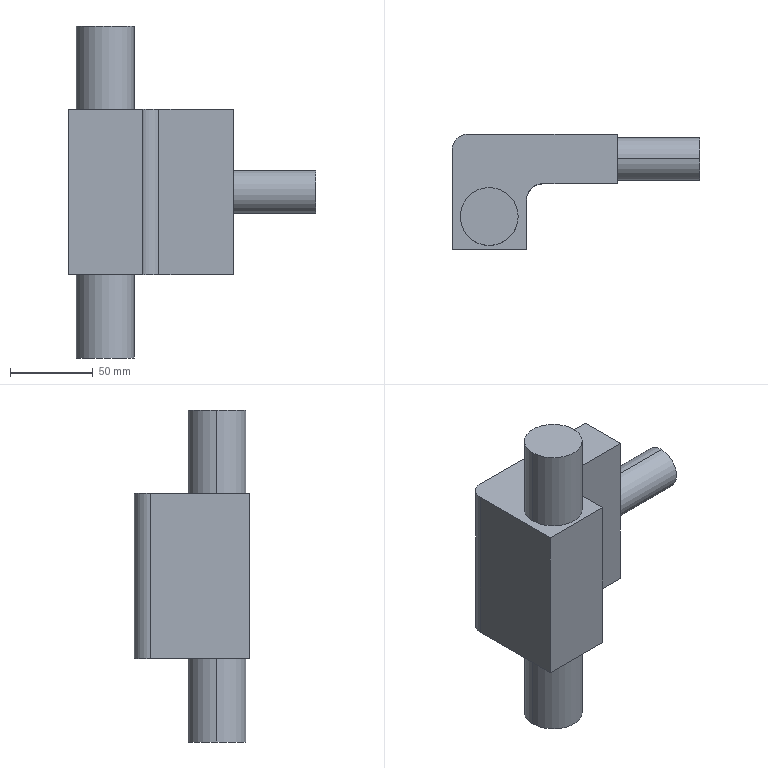Part | SolidWorks | features Revolution 3, Extrusion 1, Fillet 1, ICE 1 | 1 solid | 19 faces | box 150 x 70 x 200.87 mm | volume 603595 mm3 | plane 11 | cylinder 8 | commonest cylinder face diameters 35 x4 20 x2 26 x2
STEP:
#1=CARTESIAN_POINT('',(-17.5,0.,100.435));
#2=VERTEX_POINT('',#1);
#3=CARTESIAN_POINT('',(17.5,0.,100.435));
#4=VERTEX_POINT('',#3);
#5=CARTESIAN_POINT('',(0.,0.,100.435));
#6=DIRECTION('',(0.,0.,-1.));
#7=DIRECTION('',(-1.,0.,0.));
#8=AXIS2_PLACEMENT_3D('',#5,#6,#7);
#9=CIRCLE('',#8,17.5);
#10=EDGE_CURVE('',#2,#4,#9,.T.);
#11=ORIENTED_EDGE('',*,*,#10,.T.);
#12=CARTESIAN_POINT('',(17.5,0.,50.));
#13=VERTEX_POINT('',#12);
#14=CARTESIAN_POINT('',(17.5,0.,100.435));
#15=DIRECTION('',(0.,0.,-1.));
#16=VECTOR('',#15,1000.);
#17=LINE('',#14,#16);
#18=EDGE_CURVE('',#4,#13,#17,.T.);
#19=ORIENTED_EDGE('',*,*,#18,.T.);
#20=CARTESIAN_POINT('',(-17.5,0.,50.));
#21=VERTEX_POINT('',#20);
#22=CARTESIAN_POINT('',(0.,0.,50.));
#23=DIRECTION('',(0.,0.,1.));
#24=DIRECTION('',(1.,0.,0.));
#25=AXIS2_PLACEMENT_3D('',#22,#23,#24);
#26=CIRCLE('',#25,17.5);
#27=EDGE_CURVE('',#13,#21,#26,.T.);
#28=ORIENTED_EDGE('',*,*,#27,.T.);
#29=CARTESIAN_POINT('',(-17.5,0.,100.435));
#30=DIRECTION('',(0.,0.,-1.));
#31=VECTOR('',#30,1000.);
#32=LINE('',#29,#31);
#33=EDGE_CURVE('',#2,#21,#32,.T.);
#34=ORIENTED_EDGE('',*,*,#33,.F.);
#35=EDGE_LOOP('',(#11,#19,#28,#34));
#36=FACE_OUTER_BOUND('',#35,.T.);
#37=CARTESIAN_POINT('',(0.,0.,100.435));
#38=DIRECTION('',(0.,0.,-1.));
#39=DIRECTION('',(-1.,0.,0.));
#40=AXIS2_PLACEMENT_3D('',#37,#38,#39);
#41=CYLINDRICAL_SURFACE('',#40,17.5);
#42=ADVANCED_FACE('',(#36),#41,.T.);
#43=CARTESIAN_POINT('',(-17.5,0.,-50.));
#44=VERTEX_POINT('',#43);
#45=CARTESIAN_POINT('',(17.5,0.,-50.));
#46=VERTEX_POINT('',#45);
#47=CARTESIAN_POINT('',(0.,0.,-50.));
#48=DIRECTION('',(0.,0.,-1.));
#49=DIRECTION('',(-1.,0.,0.));
#50=AXIS2_PLACEMENT_3D('',#47,#48,#49);
#51=CIRCLE('',#50,17.5);
#52=EDGE_CURVE('',#44,#46,#51,.T.);
#53=ORIENTED_EDGE('',*,*,#52,.T.);
#54=CARTESIAN_POINT('',(17.5,0.,-100.435));
#55=VERTEX_POINT('',#54);
#56=CARTESIAN_POINT('',(17.5,0.,-50.));
#57=DIRECTION('',(0.,0.,-1.));
#58=VECTOR('',#57,1000.);
#59=LINE('',#56,#58);
#60=EDGE_CURVE('',#46,#55,#59,.T.);
#61=ORIENTED_EDGE('',*,*,#60,.T.);
#62=CARTESIAN_POINT('',(-17.5,0.,-100.435));
#63=VERTEX_POINT('',#62);
#64=CARTESIAN_POINT('',(0.,0.,-100.435));
#65=DIRECTION('',(0.,0.,-1.));
#66=DIRECTION('',(-1.,0.,0.));
#67=AXIS2_PLACEMENT_3D('',#64,#65,#66);
#68=CIRCLE('',#67,17.5);
#69=EDGE_CURVE('',#63,#55,#68,.T.);
#70=ORIENTED_EDGE('',*,*,#69,.F.);
#71=CARTESIAN_POINT('',(-17.5,0.,-50.));
#72=DIRECTION('',(0.,0.,-1.));
#73=VECTOR('',#72,1000.);
#74=LINE('',#71,#73);
#75=EDGE_CURVE('',#44,#63,#74,.T.);
#76=ORIENTED_EDGE('',*,*,#75,.F.);
#77=EDGE_LOOP('',(#53,#61,#70,#76));
#78=FACE_OUTER_BOUND('',#77,.T.);
#79=CARTESIAN_POINT('',(0.,0.,-50.));
#80=DIRECTION('',(0.,0.,-1.));
#81=DIRECTION('',(-1.,0.,0.));
#82=AXIS2_PLACEMENT_3D('',#79,#80,#81);
#83=CYLINDRICAL_SURFACE('',#82,17.5);
#84=ADVANCED_FACE('',(#78),#83,.T.);
#85=CARTESIAN_POINT('',(127.5,35.,13.));
#86=VERTEX_POINT('',#85);
#87=CARTESIAN_POINT('',(127.5,35.,-13.));
#88=VERTEX_POINT('',#87);
#89=CARTESIAN_POINT('',(127.5,35.,0.));
#90=DIRECTION('',(-1.,0.,0.));
#91=DIRECTION('',(0.,0.,1.));
#92=AXIS2_PLACEMENT_3D('',#89,#90,#91);
#93=CIRCLE('',#92,13.);
#94=EDGE_CURVE('',#86,#88,#93,.T.);
#95=ORIENTED_EDGE('',*,*,#94,.T.);
#96=CARTESIAN_POINT('',(77.5,35.,-13.));
#97=VERTEX_POINT('',#96);
#98=CARTESIAN_POINT('',(127.5,35.,-13.));
#99=DIRECTION('',(-1.,0.,0.));
#100=VECTOR('',#99,1000.);
#101=LINE('',#98,#100);
#102=EDGE_CURVE('',#88,#97,#101,.T.);
#103=ORIENTED_EDGE('',*,*,#102,.T.);
#104=CARTESIAN_POINT('',(77.5,35.,13.));
#105=VERTEX_POINT('',#104);
#106=CARTESIAN_POINT('',(77.5,35.,0.));
#107=DIRECTION('',(-1.,0.,0.));
#108=DIRECTION('',(0.,0.,1.));
#109=AXIS2_PLACEMENT_3D('',#106,#107,#108);
#110=CIRCLE('',#109,13.);
#111=EDGE_CURVE('',#105,#97,#110,.T.);
#112=ORIENTED_EDGE('',*,*,#111,.F.);
#113=CARTESIAN_POINT('',(127.5,35.,13.));
#114=DIRECTION('',(-1.,0.,0.));
#115=VECTOR('',#114,1000.);
#116=LINE('',#113,#115);
#117=EDGE_CURVE('',#86,#105,#116,.T.);
#118=ORIENTED_EDGE('',*,*,#117,.F.);
#119=EDGE_LOOP('',(#95,#103,#112,#118));
#120=FACE_OUTER_BOUND('',#119,.T.);
#121=CARTESIAN_POINT('',(127.5,35.,0.));
#122=DIRECTION('',(-1.,0.,0.));
#123=DIRECTION('',(0.,0.,1.));
#124=AXIS2_PLACEMENT_3D('',#121,#122,#123);
#125=CYLINDRICAL_SURFACE('',#124,13.);
#126=ADVANCED_FACE('',(#120),#125,.T.);
#127=CARTESIAN_POINT('',(-22.5,40.,50.));
#128=VERTEX_POINT('',#127);
#129=CARTESIAN_POINT('',(-22.5,-20.,50.));
#130=VERTEX_POINT('',#129);
#131=CARTESIAN_POINT('',(-22.5,50.,50.));
#132=DIRECTION('',(0.,-1.,0.));
#133=VECTOR('',#132,1000.);
#134=LINE('',#131,#133);
#135=EDGE_CURVE('',#128,#130,#134,.T.);
#136=ORIENTED_EDGE('',*,*,#135,.F.);
#137=CARTESIAN_POINT('',(-22.5,40.,-50.));
#138=VERTEX_POINT('',#137);
#139=CARTESIAN_POINT('',(-22.5,40.,-50.));
#140=DIRECTION('',(0.,0.,-1.));
#141=VECTOR('',#140,1000.);
#142=LINE('',#139,#141);
#143=EDGE_CURVE('',#128,#138,#142,.T.);
#144=ORIENTED_EDGE('',*,*,#143,.T.);
#145=CARTESIAN_POINT('',(-22.5,-20.,-50.));
#146=VERTEX_POINT('',#145);
#147=CARTESIAN_POINT('',(-22.5,50.,-50.));
#148=DIRECTION('',(0.,-1.,0.));
#149=VECTOR('',#148,1000.);
#150=LINE('',#147,#149);
#151=EDGE_CURVE('',#138,#146,#150,.T.);
#152=ORIENTED_EDGE('',*,*,#151,.T.);
#153=CARTESIAN_POINT('',(-22.5,-20.,50.));
#154=DIRECTION('',(0.,0.,-1.));
#155=VECTOR('',#154,1000.);
#156=LINE('',#153,#155);
#157=EDGE_CURVE('',#130,#146,#156,.T.);
#158=ORIENTED_EDGE('',*,*,#157,.F.);
#159=EDGE_LOOP('',(#136,#144,#152,#158));
#160=FACE_OUTER_BOUND('',#159,.T.);
#161=CARTESIAN_POINT('',(-22.5,50.,50.));
#162=DIRECTION('',(-1.,0.,0.));
#163=DIRECTION('',(0.,0.,1.));
#164=AXIS2_PLACEMENT_3D('',#161,#162,#163);
#165=PLANE('',#164);
#166=ADVANCED_FACE('',(#160),#165,.T.);
#167=CARTESIAN_POINT('',(0.,0.,50.));
#168=DIRECTION('',(0.,0.,1.));
#169=DIRECTION('',(1.,0.,0.));
#170=AXIS2_PLACEMENT_3D('',#167,#168,#169);
#171=CIRCLE('',#170,17.5);
#172=EDGE_CURVE('',#21,#13,#171,.T.);
#173=ORIENTED_EDGE('',*,*,#172,.F.);
#174=ORIENTED_EDGE('',*,*,#27,.F.);
#175=EDGE_LOOP('',(#173,#174));
#176=FACE_BOUND('',#175,.T.);
#177=CARTESIAN_POINT('',(77.5,50.,50.));
#178=VERTEX_POINT('',#177);
#179=CARTESIAN_POINT('',(-12.5,50.,50.));
#180=VERTEX_POINT('',#179);
#181=CARTESIAN_POINT('',(77.5,50.,50.));
#182=DIRECTION('',(-1.,0.,0.));
#183=VECTOR('',#182,1000.);
#184=LINE('',#181,#183);
#185=EDGE_CURVE('',#178,#180,#184,.T.);
#186=ORIENTED_EDGE('',*,*,#185,.T.);
#187=CARTESIAN_POINT('',(-12.5,40.,50.));
#188=DIRECTION('',(0.,0.,1.));
#189=DIRECTION('',(1.,0.,0.));
#190=AXIS2_PLACEMENT_3D('',#187,#188,#189);
#191=CIRCLE('',#190,10.);
#192=EDGE_CURVE('',#180,#128,#191,.T.);
#193=ORIENTED_EDGE('',*,*,#192,.T.);
#194=ORIENTED_EDGE('',*,*,#135,.T.);
#195=CARTESIAN_POINT('',(22.5,-20.,50.));
#196=VERTEX_POINT('',#195);
#197=CARTESIAN_POINT('',(77.5,-20.,50.));
#198=DIRECTION('',(-1.,0.,0.));
#199=VECTOR('',#198,1000.);
#200=LINE('',#197,#199);
#201=EDGE_CURVE('',#196,#130,#200,.T.);
#202=ORIENTED_EDGE('',*,*,#201,.F.);
#203=CARTESIAN_POINT('',(22.5,10.,50.));
#204=VERTEX_POINT('',#203);
#205=CARTESIAN_POINT('',(22.5,-20.,50.));
#206=DIRECTION('',(0.,1.,0.));
#207=VECTOR('',#206,1000.);
#208=LINE('',#205,#207);
#209=EDGE_CURVE('',#196,#204,#208,.T.);
#210=ORIENTED_EDGE('',*,*,#209,.T.);
#211=CARTESIAN_POINT('',(32.5,20.,50.));
#212=VERTEX_POINT('',#211);
#213=CARTESIAN_POINT('',(32.5,10.,50.));
#214=DIRECTION('',(0.,0.,-1.));
#215=DIRECTION('',(1.,0.,0.));
#216=AXIS2_PLACEMENT_3D('',#213,#214,#215);
#217=CIRCLE('',#216,10.);
#218=EDGE_CURVE('',#204,#212,#217,.T.);
#219=ORIENTED_EDGE('',*,*,#218,.T.);
#220=CARTESIAN_POINT('',(77.5,20.,50.));
#221=VERTEX_POINT('',#220);
#222=CARTESIAN_POINT('',(22.5,20.,50.));
#223=DIRECTION('',(1.,0.,0.));
#224=VECTOR('',#223,1000.);
#225=LINE('',#222,#224);
#226=EDGE_CURVE('',#212,#221,#225,.T.);
#227=ORIENTED_EDGE('',*,*,#226,.T.);
#228=CARTESIAN_POINT('',(77.5,50.,50.));
#229=DIRECTION('',(0.,-1.,0.));
#230=VECTOR('',#229,1000.);
#231=LINE('',#228,#230);
#232=EDGE_CURVE('',#178,#221,#231,.T.);
#233=ORIENTED_EDGE('',*,*,#232,.F.);
#234=EDGE_LOOP('',(#186,#193,#194,#202,#210,#219,#227,#233));
#235=FACE_OUTER_BOUND('',#234,.T.);
#236=CARTESIAN_POINT('',(77.5,50.,50.));
#237=DIRECTION('',(0.,0.,1.));
#238=DIRECTION('',(1.,0.,0.));
#239=AXIS2_PLACEMENT_3D('',#236,#237,#238);
#240=PLANE('',#239);
#241=ADVANCED_FACE('',(#176,#235),#240,.T.);
#242=ORIENTED_EDGE('',*,*,#111,.T.);
#243=CARTESIAN_POINT('',(77.5,35.,0.));
#244=DIRECTION('',(-1.,0.,0.));
#245=DIRECTION('',(0.,0.,1.));
#246=AXIS2_PLACEMENT_3D('',#243,#244,#245);
#247=CIRCLE('',#246,13.);
#248=EDGE_CURVE('',#97,#105,#247,.T.);
#249=ORIENTED_EDGE('',*,*,#248,.T.);
#250=EDGE_LOOP('',(#242,#249));
#251=FACE_BOUND('',#250,.T.);
#252=CARTESIAN_POINT('',(77.5,20.,-50.));
#253=VERTEX_POINT('',#252);
#254=CARTESIAN_POINT('',(77.5,20.,50.));
#255=DIRECTION('',(0.,0.,-1.));
#256=VECTOR('',#255,1000.);
#257=LINE('',#254,#256);
#258=EDGE_CURVE('',#221,#253,#257,.T.);
#259=ORIENTED_EDGE('',*,*,#258,.T.);
#260=CARTESIAN_POINT('',(77.5,50.,-50.));
#261=VERTEX_POINT('',#260);
#262=CARTESIAN_POINT('',(77.5,50.,-50.));
#263=DIRECTION('',(0.,-1.,0.));
#264=VECTOR('',#263,1000.);
#265=LINE('',#262,#264);
#266=EDGE_CURVE('',#261,#253,#265,.T.);
#267=ORIENTED_EDGE('',*,*,#266,.F.);
#268=CARTESIAN_POINT('',(77.5,50.,-50.));
#269=DIRECTION('',(0.,0.,1.));
#270=VECTOR('',#269,1000.);
#271=LINE('',#268,#270);
#272=EDGE_CURVE('',#261,#178,#271,.T.);
#273=ORIENTED_EDGE('',*,*,#272,.T.);
#274=ORIENTED_EDGE('',*,*,#232,.T.);
#275=EDGE_LOOP('',(#259,#267,#273,#274));
#276=FACE_OUTER_BOUND('',#275,.T.);
#277=CARTESIAN_POINT('',(77.5,50.,-50.));
#278=DIRECTION('',(1.,0.,0.));
#279=DIRECTION('',(0.,0.,-1.));
#280=AXIS2_PLACEMENT_3D('',#277,#278,#279);
#281=PLANE('',#280);
#282=ADVANCED_FACE('',(#251,#276),#281,.T.);
#283=ORIENTED_EDGE('',*,*,#52,.F.);
#284=CARTESIAN_POINT('',(0.,0.,-50.));
#285=DIRECTION('',(0.,0.,-1.));
#286=DIRECTION('',(-1.,0.,0.));
#287=AXIS2_PLACEMENT_3D('',#284,#285,#286);
#288=CIRCLE('',#287,17.5);
#289=EDGE_CURVE('',#46,#44,#288,.T.);
#290=ORIENTED_EDGE('',*,*,#289,.F.);
#291=EDGE_LOOP('',(#283,#290));
#292=FACE_BOUND('',#291,.T.);
#293=ORIENTED_EDGE('',*,*,#151,.F.);
#294=CARTESIAN_POINT('',(-12.5,50.,-50.));
#295=VERTEX_POINT('',#294);
#296=CARTESIAN_POINT('',(-12.5,40.,-50.));
#297=DIRECTION('',(0.,0.,-1.));
#298=DIRECTION('',(-1.,0.,0.));
#299=AXIS2_PLACEMENT_3D('',#296,#297,#298);
#300=CIRCLE('',#299,10.);
#301=EDGE_CURVE('',#138,#295,#300,.T.);
#302=ORIENTED_EDGE('',*,*,#301,.T.);
#303=CARTESIAN_POINT('',(-22.5,50.,-50.));
#304=DIRECTION('',(1.,0.,0.));
#305=VECTOR('',#304,1000.);
#306=LINE('',#303,#305);
#307=EDGE_CURVE('',#295,#261,#306,.T.);
#308=ORIENTED_EDGE('',*,*,#307,.T.);
#309=ORIENTED_EDGE('',*,*,#266,.T.);
#310=CARTESIAN_POINT('',(32.5,20.,-50.));
#311=VERTEX_POINT('',#310);
#312=CARTESIAN_POINT('',(22.5,20.,-50.));
#313=DIRECTION('',(1.,0.,0.));
#314=VECTOR('',#313,1000.);
#315=LINE('',#312,#314);
#316=EDGE_CURVE('',#311,#253,#315,.T.);
#317=ORIENTED_EDGE('',*,*,#316,.F.);
#318=CARTESIAN_POINT('',(22.5,10.,-50.));
#319=VERTEX_POINT('',#318);
#320=CARTESIAN_POINT('',(32.5,10.,-50.));
#321=DIRECTION('',(0.,0.,1.));
#322=DIRECTION('',(-1.,0.,0.));
#323=AXIS2_PLACEMENT_3D('',#320,#321,#322);
#324=CIRCLE('',#323,10.);
#325=EDGE_CURVE('',#311,#319,#324,.T.);
#326=ORIENTED_EDGE('',*,*,#325,.T.);
#327=CARTESIAN_POINT('',(22.5,-20.,-50.));
#328=VERTEX_POINT('',#327);
#329=CARTESIAN_POINT('',(22.5,-20.,-50.));
#330=DIRECTION('',(0.,1.,0.));
#331=VECTOR('',#330,1000.);
#332=LINE('',#329,#331);
#333=EDGE_CURVE('',#328,#319,#332,.T.);
#334=ORIENTED_EDGE('',*,*,#333,.F.);
#335=CARTESIAN_POINT('',(-22.5,-20.,-50.));
#336=DIRECTION('',(1.,0.,0.));
#337=VECTOR('',#336,1000.);
#338=LINE('',#335,#337);
#339=EDGE_CURVE('',#146,#328,#338,.T.);
#340=ORIENTED_EDGE('',*,*,#339,.F.);
#341=EDGE_LOOP('',(#293,#302,#308,#309,#317,#326,#334,#340));
#342=FACE_OUTER_BOUND('',#341,.T.);
#343=CARTESIAN_POINT('',(-22.5,50.,-50.));
#344=DIRECTION('',(0.,0.,-1.));
#345=DIRECTION('',(-1.,0.,0.));
#346=AXIS2_PLACEMENT_3D('',#343,#344,#345);
#347=PLANE('',#346);
#348=ADVANCED_FACE('',(#292,#342),#347,.T.);
#349=ORIENTED_EDGE('',*,*,#307,.F.);
#350=CARTESIAN_POINT('',(-12.5,50.,50.));
#351=DIRECTION('',(0.,0.,1.));
#352=VECTOR('',#351,1000.);
#353=LINE('',#350,#352);
#354=EDGE_CURVE('',#295,#180,#353,.T.);
#355=ORIENTED_EDGE('',*,*,#354,.T.);
#356=ORIENTED_EDGE('',*,*,#185,.F.);
#357=ORIENTED_EDGE('',*,*,#272,.F.);
#358=EDGE_LOOP('',(#349,#355,#356,#357));
#359=FACE_OUTER_BOUND('',#358,.T.);
#360=CARTESIAN_POINT('',(0.,50.,0.));
#361=DIRECTION('',(0.,-1.,0.));
#362=DIRECTION('',(0.,0.,-1.));
#363=AXIS2_PLACEMENT_3D('',#360,#361,#362);
#364=PLANE('',#363);
#365=ADVANCED_FACE('',(#359),#364,.F.);
#366=CARTESIAN_POINT('',(22.5,-20.,50.));
#367=DIRECTION('',(0.,0.,-1.));
#368=VECTOR('',#367,1000.);
#369=LINE('',#366,#368);
#370=EDGE_CURVE('',#196,#328,#369,.T.);
#371=ORIENTED_EDGE('',*,*,#370,.F.);
#372=ORIENTED_EDGE('',*,*,#201,.T.);
#373=ORIENTED_EDGE('',*,*,#157,.T.);
#374=ORIENTED_EDGE('',*,*,#339,.T.);
#375=EDGE_LOOP('',(#371,#372,#373,#374));
#376=FACE_OUTER_BOUND('',#375,.T.);
#377=CARTESIAN_POINT('',(0.,-20.,0.));
#378=DIRECTION('',(0.,-1.,0.));
#379=DIRECTION('',(0.,0.,-1.));
#380=AXIS2_PLACEMENT_3D('',#377,#378,#379);
#381=PLANE('',#380);
#382=ADVANCED_FACE('',(#376),#381,.T.);
#383=ORIENTED_EDGE('',*,*,#226,.F.);
#384=CARTESIAN_POINT('',(32.5,20.,-50.));
#385=DIRECTION('',(0.,0.,-1.));
#386=VECTOR('',#385,1000.);
#387=LINE('',#384,#386);
#388=EDGE_CURVE('',#212,#311,#387,.T.);
#389=ORIENTED_EDGE('',*,*,#388,.T.);
#390=ORIENTED_EDGE('',*,*,#316,.T.);
#391=ORIENTED_EDGE('',*,*,#258,.F.);
#392=EDGE_LOOP('',(#383,#389,#390,#391));
#393=FACE_OUTER_BOUND('',#392,.T.);
#394=CARTESIAN_POINT('',(22.5,20.,50.));
#395=DIRECTION('',(0.,1.,0.));
#396=DIRECTION('',(0.,0.,1.));
#397=AXIS2_PLACEMENT_3D('',#394,#395,#396);
#398=PLANE('',#397);
#399=ADVANCED_FACE('',(#393),#398,.F.);
#400=ORIENTED_EDGE('',*,*,#333,.T.);
#401=CARTESIAN_POINT('',(22.5,10.,50.));
#402=DIRECTION('',(0.,0.,1.));
#403=VECTOR('',#402,1000.);
#404=LINE('',#401,#403);
#405=EDGE_CURVE('',#319,#204,#404,.T.);
#406=ORIENTED_EDGE('',*,*,#405,.T.);
#407=ORIENTED_EDGE('',*,*,#209,.F.);
#408=ORIENTED_EDGE('',*,*,#370,.T.);
#409=EDGE_LOOP('',(#400,#406,#407,#408));
#410=FACE_OUTER_BOUND('',#409,.T.);
#411=CARTESIAN_POINT('',(22.5,-20.,50.));
#412=DIRECTION('',(-1.,0.,0.));
#413=DIRECTION('',(0.,0.,1.));
#414=AXIS2_PLACEMENT_3D('',#411,#412,#413);
#415=PLANE('',#414);
#416=ADVANCED_FACE('',(#410),#415,.F.);
#417=ORIENTED_EDGE('',*,*,#102,.F.);
#418=CARTESIAN_POINT('',(127.5,35.,0.));
#419=DIRECTION('',(-1.,0.,0.));
#420=DIRECTION('',(0.,0.,1.));
#421=AXIS2_PLACEMENT_3D('',#418,#419,#420);
#422=CIRCLE('',#421,13.);
#423=EDGE_CURVE('',#88,#86,#422,.T.);
#424=ORIENTED_EDGE('',*,*,#423,.T.);
#425=ORIENTED_EDGE('',*,*,#117,.T.);
#426=ORIENTED_EDGE('',*,*,#248,.F.);
#427=EDGE_LOOP('',(#417,#424,#425,#426));
#428=FACE_OUTER_BOUND('',#427,.T.);
#429=CARTESIAN_POINT('',(127.5,35.,0.));
#430=DIRECTION('',(-1.,0.,0.));
#431=DIRECTION('',(0.,0.,1.));
#432=AXIS2_PLACEMENT_3D('',#429,#430,#431);
#433=CYLINDRICAL_SURFACE('',#432,13.);
#434=ADVANCED_FACE('',(#428),#433,.T.);
#435=ORIENTED_EDGE('',*,*,#94,.F.);
#436=ORIENTED_EDGE('',*,*,#423,.F.);
#437=EDGE_LOOP('',(#435,#436));
#438=FACE_OUTER_BOUND('',#437,.T.);
#439=CARTESIAN_POINT('',(127.5,48.,0.));
#440=DIRECTION('',(1.,0.,0.));
#441=DIRECTION('',(0.,0.,-1.));
#442=AXIS2_PLACEMENT_3D('',#439,#440,#441);
#443=PLANE('',#442);
#444=ADVANCED_FACE('',(#438),#443,.T.);
#445=ORIENTED_EDGE('',*,*,#60,.F.);
#446=ORIENTED_EDGE('',*,*,#289,.T.);
#447=ORIENTED_EDGE('',*,*,#75,.T.);
#448=CARTESIAN_POINT('',(0.,0.,-100.435));
#449=DIRECTION('',(0.,0.,-1.));
#450=DIRECTION('',(-1.,0.,0.));
#451=AXIS2_PLACEMENT_3D('',#448,#449,#450);
#452=CIRCLE('',#451,17.5);
#453=EDGE_CURVE('',#55,#63,#452,.T.);
#454=ORIENTED_EDGE('',*,*,#453,.F.);
#455=EDGE_LOOP('',(#445,#446,#447,#454));
#456=FACE_OUTER_BOUND('',#455,.T.);
#457=CARTESIAN_POINT('',(0.,0.,-50.));
#458=DIRECTION('',(0.,0.,-1.));
#459=DIRECTION('',(-1.,0.,0.));
#460=AXIS2_PLACEMENT_3D('',#457,#458,#459);
#461=CYLINDRICAL_SURFACE('',#460,17.5);
#462=ADVANCED_FACE('',(#456),#461,.T.);
#463=ORIENTED_EDGE('',*,*,#69,.T.);
#464=ORIENTED_EDGE('',*,*,#453,.T.);
#465=EDGE_LOOP('',(#463,#464));
#466=FACE_OUTER_BOUND('',#465,.T.);
#467=CARTESIAN_POINT('',(0.,0.,-100.435));
#468=DIRECTION('',(0.,0.,-1.));
#469=DIRECTION('',(-1.,0.,0.));
#470=AXIS2_PLACEMENT_3D('',#467,#468,#469);
#471=PLANE('',#470);
#472=ADVANCED_FACE('',(#466),#471,.T.);
#473=ORIENTED_EDGE('',*,*,#18,.F.);
#474=CARTESIAN_POINT('',(0.,0.,100.435));
#475=DIRECTION('',(0.,0.,-1.));
#476=DIRECTION('',(-1.,0.,0.));
#477=AXIS2_PLACEMENT_3D('',#474,#475,#476);
#478=CIRCLE('',#477,17.5);
#479=EDGE_CURVE('',#4,#2,#478,.T.);
#480=ORIENTED_EDGE('',*,*,#479,.T.);
#481=ORIENTED_EDGE('',*,*,#33,.T.);
#482=ORIENTED_EDGE('',*,*,#172,.T.);
#483=EDGE_LOOP('',(#473,#480,#481,#482));
#484=FACE_OUTER_BOUND('',#483,.T.);
#485=CARTESIAN_POINT('',(0.,0.,100.435));
#486=DIRECTION('',(0.,0.,-1.));
#487=DIRECTION('',(-1.,0.,0.));
#488=AXIS2_PLACEMENT_3D('',#485,#486,#487);
#489=CYLINDRICAL_SURFACE('',#488,17.5);
#490=ADVANCED_FACE('',(#484),#489,.T.);
#491=ORIENTED_EDGE('',*,*,#10,.F.);
#492=ORIENTED_EDGE('',*,*,#479,.F.);
#493=EDGE_LOOP('',(#491,#492));
#494=FACE_OUTER_BOUND('',#493,.T.);
#495=CARTESIAN_POINT('',(17.5,0.,100.435));
#496=DIRECTION('',(0.,0.,1.));
#497=DIRECTION('',(1.,0.,0.));
#498=AXIS2_PLACEMENT_3D('',#495,#496,#497);
#499=PLANE('',#498);
#500=ADVANCED_FACE('',(#494),#499,.T.);
#501=ORIENTED_EDGE('',*,*,#192,.F.);
#502=ORIENTED_EDGE('',*,*,#354,.F.);
#503=ORIENTED_EDGE('',*,*,#301,.F.);
#504=ORIENTED_EDGE('',*,*,#143,.F.);
#505=EDGE_LOOP('',(#501,#502,#503,#504));
#506=FACE_OUTER_BOUND('',#505,.T.);
#507=CARTESIAN_POINT('',(-12.5,40.,50.));
#508=DIRECTION('',(0.,0.,1.));
#509=DIRECTION('',(1.,0.,0.));
#510=AXIS2_PLACEMENT_3D('',#507,#508,#509);
#511=CYLINDRICAL_SURFACE('',#510,10.);
#512=ADVANCED_FACE('',(#506),#511,.T.);
#513=ORIENTED_EDGE('',*,*,#218,.F.);
#514=ORIENTED_EDGE('',*,*,#405,.F.);
#515=ORIENTED_EDGE('',*,*,#325,.F.);
#516=ORIENTED_EDGE('',*,*,#388,.F.);
#517=EDGE_LOOP('',(#513,#514,#515,#516));
#518=FACE_OUTER_BOUND('',#517,.T.);
#519=CARTESIAN_POINT('',(32.5,10.,50.));
#520=DIRECTION('',(0.,0.,1.));
#521=DIRECTION('',(1.,0.,0.));
#522=AXIS2_PLACEMENT_3D('',#519,#520,#521);
#523=CYLINDRICAL_SURFACE('',#522,10.);
#524=ADVANCED_FACE('',(#518),#523,.F.);
#525=CLOSED_SHELL('',(#42,#84,#126,#166,#241,#282,#348,#365,#382,#399,#416,#434,#444,#462,#472,#490,#500,#512,#524));
#526=MANIFOLD_SOLID_BREP('',#525);
#527=CARTESIAN_POINT('',(0.,0.,0.));
#528=DIRECTION('',(0.,0.,1.));
#529=DIRECTION('',(1.,0.,0.));
#530=AXIS2_PLACEMENT_3D('',#527,#528,#529);
#531=(LENGTH_UNIT()NAMED_UNIT(*)SI_UNIT(.MILLI.,.METRE.));
#532=UNCERTAINTY_MEASURE_WITH_UNIT(LENGTH_MEASURE(0.00001),#531,'','');
#533=(NAMED_UNIT(*)PLANE_ANGLE_UNIT()SI_UNIT($,.RADIAN.));
#534=(NAMED_UNIT(*)SI_UNIT($,.STERADIAN.)SOLID_ANGLE_UNIT());
#535=(GEOMETRIC_REPRESENTATION_CONTEXT(3)GLOBAL_UNCERTAINTY_ASSIGNED_CONTEXT((#532))GLOBAL_UNIT_ASSIGNED_CONTEXT((#531,#533,#534))REPRESENTATION_CONTEXT('',''));
#536=ADVANCED_BREP_SHAPE_REPRESENTATION('',(#526,#530),#535);